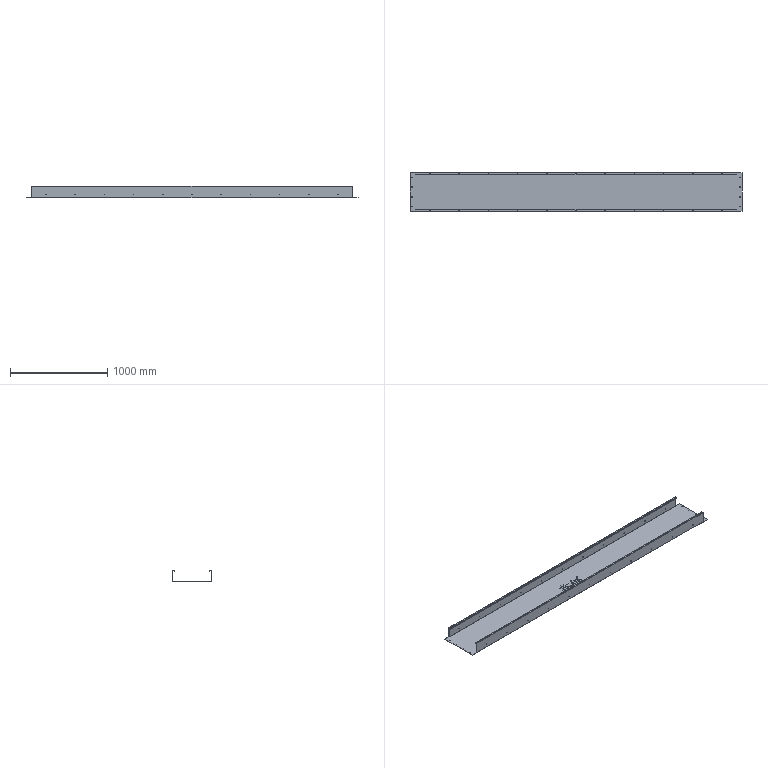Part | STEP file | TS-S77 TBD | 1 solid | 282 faces | box 3411 x 400 x 120 mm | volume 4608204 mm3 | plane 133 | cylinder 116 | spline 33 | commonest cylinder face diameters 5.4 x88 7 x16 0.4 x6 4.4 x6